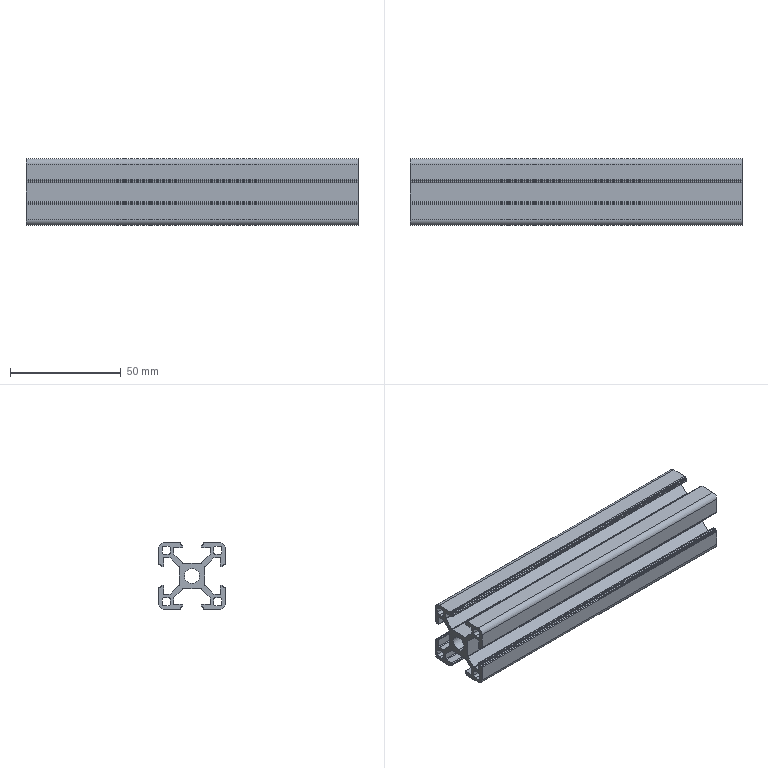Part | STEP file | MK-8-3030-L-00 profile 3030 standard type 150mm | 1 solid | 155 faces | box 150 x 30 x 30 mm | volume 48990 mm3 | plane 78 | cylinder 77 | commonest cylinder face diameters 0.6 x55 2 x16 5 x4 6.8 x2